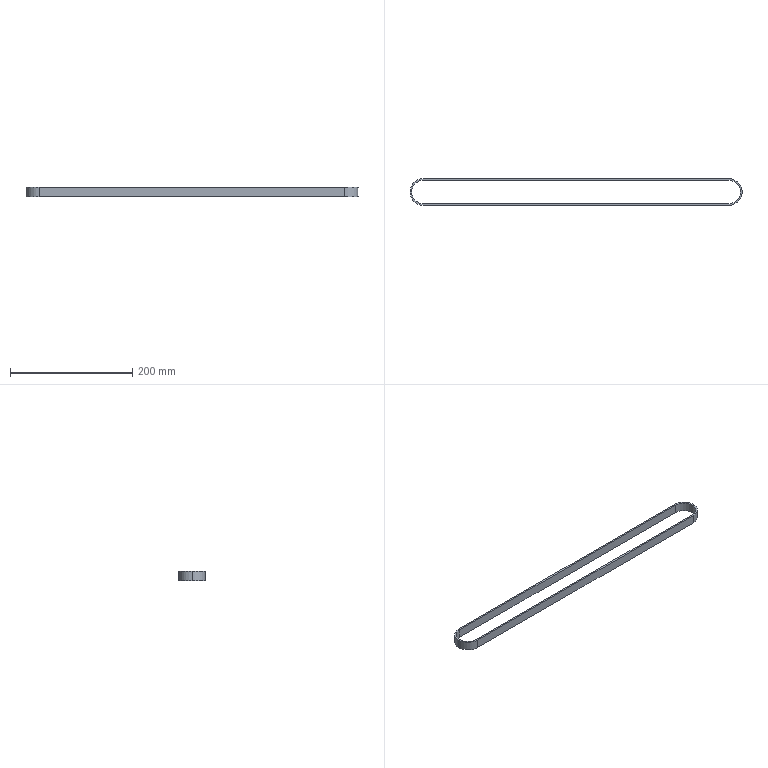Part | STEP file | Belt 1-2^ double-tube high-torque assembly | 1 solid | 12 faces | box 543.89 x 43.89 x 15 mm | volume 44395 mm3 | cylinder 6 | plane 6 | commonest cylinder face diameters 38.65 x3 43.89 x3
STEP:
#1=CARTESIAN_POINT('',(0.,0.,0.));
#2=DIRECTION('',(0.,0.,1.));
#3=DIRECTION('',(1.,0.,0.));
#4=AXIS2_PLACEMENT_3D('',#1,#2,#3);
#5=CARTESIAN_POINT('',(-14.086,14.168,15.));
#6=VERTEX_POINT('',#5);
#7=CARTESIAN_POINT('',(-14.086,14.168,0.));
#8=VERTEX_POINT('',#7);
#9=CARTESIAN_POINT('',(-14.086,14.168,15.));
#10=DIRECTION('',(0.,0.,-1.));
#11=VECTOR('',#10,1.);
#12=LINE('',#9,#11);
#13=CARTESIAN_POINT('',(-14.086,-5.157,15.));
#14=DIRECTION('',(0.,0.,-1.));
#15=DIRECTION('',(-1.,0.,0.));
#16=AXIS2_PLACEMENT_3D('',#13,#14,#15);
#17=CYLINDRICAL_SURFACE('',#16,19.325);
#18=CARTESIAN_POINT('',(1.571,0.));
#19=DIRECTION('',(0.,1.));
#20=VECTOR('',#19,1.);
#21=LINE('',#18,#20);
#22=(GEOMETRIC_REPRESENTATION_CONTEXT(2)PARAMETRIC_REPRESENTATION_CONTEXT()REPRESENTATION_CONTEXT('',''));
#23=DEFINITIONAL_REPRESENTATION('',(#21),#22);
#24=PCURVE('',#17,#23);
#25=CARTESIAN_POINT('',(-14.086,14.168,15.));
#26=DIRECTION('',(0.,1.,0.));
#27=DIRECTION('',(-1.,0.,0.));
#28=AXIS2_PLACEMENT_3D('',#25,#26,#27);
#29=PLANE('',#28);
#30=CARTESIAN_POINT('',(0.,0.));
#31=DIRECTION('',(0.,-1.));
#32=VECTOR('',#31,1.);
#33=LINE('',#30,#32);
#34=(GEOMETRIC_REPRESENTATION_CONTEXT(2)PARAMETRIC_REPRESENTATION_CONTEXT()REPRESENTATION_CONTEXT('',''));
#35=DEFINITIONAL_REPRESENTATION('',(#33),#34);
#36=PCURVE('',#29,#35);
#37=SURFACE_CURVE('',#12,(#24,#36),.PCURVE_S1.);
#38=EDGE_CURVE('',#6,#8,#37,.T.);
#39=ORIENTED_EDGE('',*,*,#38,.T.);
#40=CARTESIAN_POINT('',(-33.411,-5.157,0.));
#41=VERTEX_POINT('',#40);
#42=CARTESIAN_POINT('',(-14.086,-5.157,0.));
#43=DIRECTION('',(0.,0.,-1.));
#44=DIRECTION('',(-1.,0.,0.));
#45=AXIS2_PLACEMENT_3D('',#42,#43,#44);
#46=CIRCLE('',#45,19.325);
#47=CARTESIAN_POINT('',(0.,15.));
#48=DIRECTION('',(1.,0.));
#49=VECTOR('',#48,1.);
#50=LINE('',#47,#49);
#51=(GEOMETRIC_REPRESENTATION_CONTEXT(2)PARAMETRIC_REPRESENTATION_CONTEXT()REPRESENTATION_CONTEXT('',''));
#52=DEFINITIONAL_REPRESENTATION('',(#50),#51);
#53=PCURVE('',#17,#52);
#54=CARTESIAN_POINT('',(-14.086,-5.157,0.));
#55=DIRECTION('',(0.,0.,-1.));
#56=DIRECTION('',(-1.,0.,0.));
#57=AXIS2_PLACEMENT_3D('',#54,#55,#56);
#58=PLANE('',#57);
#59=CARTESIAN_POINT('',(0.,0.));
#60=DIRECTION('',(1.,0.));
#61=AXIS2_PLACEMENT_2D('',#59,#60);
#62=CIRCLE('',#61,19.325);
#63=(GEOMETRIC_REPRESENTATION_CONTEXT(2)PARAMETRIC_REPRESENTATION_CONTEXT()REPRESENTATION_CONTEXT('',''));
#64=DEFINITIONAL_REPRESENTATION('',(#62),#63);
#65=PCURVE('',#58,#64);
#66=SURFACE_CURVE('',#46,(#53,#65),.PCURVE_S1.);
#67=EDGE_CURVE('',#41,#8,#66,.T.);
#68=ORIENTED_EDGE('',*,*,#67,.F.);
#69=CARTESIAN_POINT('',(-33.411,-5.157,15.));
#70=VERTEX_POINT('',#69);
#71=CARTESIAN_POINT('',(-33.411,-5.157,15.));
#72=DIRECTION('',(0.,0.,-1.));
#73=VECTOR('',#72,1.);
#74=LINE('',#71,#73);
#75=CARTESIAN_POINT('',(0.,0.));
#76=DIRECTION('',(0.,1.));
#77=VECTOR('',#76,1.);
#78=LINE('',#75,#77);
#79=(GEOMETRIC_REPRESENTATION_CONTEXT(2)PARAMETRIC_REPRESENTATION_CONTEXT()REPRESENTATION_CONTEXT('',''));
#80=DEFINITIONAL_REPRESENTATION('',(#78),#79);
#81=PCURVE('',#17,#80);
#82=CARTESIAN_POINT('',(-14.086,-5.157,15.));
#83=DIRECTION('',(0.,0.,-1.));
#84=DIRECTION('',(-1.,0.,0.));
#85=AXIS2_PLACEMENT_3D('',#82,#83,#84);
#86=CYLINDRICAL_SURFACE('',#85,19.325);
#87=CARTESIAN_POINT('',(6.283,0.));
#88=DIRECTION('',(0.,1.));
#89=VECTOR('',#88,1.);
#90=LINE('',#87,#89);
#91=(GEOMETRIC_REPRESENTATION_CONTEXT(2)PARAMETRIC_REPRESENTATION_CONTEXT()REPRESENTATION_CONTEXT('',''));
#92=DEFINITIONAL_REPRESENTATION('',(#90),#91);
#93=PCURVE('',#86,#92);
#94=SURFACE_CURVE('',#74,(#81,#93),.PCURVE_S1.);
#95=EDGE_CURVE('',#70,#41,#94,.T.);
#96=ORIENTED_EDGE('',*,*,#95,.F.);
#97=CARTESIAN_POINT('',(-14.086,-5.157,15.));
#98=DIRECTION('',(0.,0.,-1.));
#99=DIRECTION('',(-1.,0.,0.));
#100=AXIS2_PLACEMENT_3D('',#97,#98,#99);
#101=CIRCLE('',#100,19.325);
#102=CARTESIAN_POINT('',(0.,0.));
#103=DIRECTION('',(1.,0.));
#104=VECTOR('',#103,1.);
#105=LINE('',#102,#104);
#106=(GEOMETRIC_REPRESENTATION_CONTEXT(2)PARAMETRIC_REPRESENTATION_CONTEXT()REPRESENTATION_CONTEXT('',''));
#107=DEFINITIONAL_REPRESENTATION('',(#105),#106);
#108=PCURVE('',#17,#107);
#109=CARTESIAN_POINT('',(-14.086,-5.157,15.));
#110=DIRECTION('',(0.,0.,-1.));
#111=DIRECTION('',(-1.,0.,0.));
#112=AXIS2_PLACEMENT_3D('',#109,#110,#111);
#113=PLANE('',#112);
#114=CARTESIAN_POINT('',(0.,0.));
#115=DIRECTION('',(1.,0.));
#116=AXIS2_PLACEMENT_2D('',#114,#115);
#117=CIRCLE('',#116,19.325);
#118=(GEOMETRIC_REPRESENTATION_CONTEXT(2)PARAMETRIC_REPRESENTATION_CONTEXT()REPRESENTATION_CONTEXT('',''));
#119=DEFINITIONAL_REPRESENTATION('',(#117),#118);
#120=PCURVE('',#113,#119);
#121=SURFACE_CURVE('',#101,(#108,#120),.PCURVE_S1.);
#122=EDGE_CURVE('',#70,#6,#121,.T.);
#123=ORIENTED_EDGE('',*,*,#122,.T.);
#124=EDGE_LOOP('',(#39,#68,#96,#123));
#125=FACE_BOUND('',#124,.F.);
#126=ADVANCED_FACE('',(#125),#17,.F.);
#127=CARTESIAN_POINT('',(-14.086,-27.102,15.));
#128=VERTEX_POINT('',#127);
#129=CARTESIAN_POINT('',(-36.031,-5.157,15.));
#130=VERTEX_POINT('',#129);
#131=CARTESIAN_POINT('',(-14.086,-5.157,15.));
#132=DIRECTION('',(0.,0.,-1.));
#133=DIRECTION('',(-1.,0.,0.));
#134=AXIS2_PLACEMENT_3D('',#131,#132,#133);
#135=CIRCLE('',#134,21.945);
#136=CARTESIAN_POINT('',(-14.086,-5.157,15.));
#137=DIRECTION('',(0.,0.,-1.));
#138=DIRECTION('',(-1.,0.,0.));
#139=AXIS2_PLACEMENT_3D('',#136,#137,#138);
#140=CYLINDRICAL_SURFACE('',#139,21.945);
#141=CARTESIAN_POINT('',(0.,0.));
#142=DIRECTION('',(1.,0.));
#143=VECTOR('',#142,1.);
#144=LINE('',#141,#143);
#145=(GEOMETRIC_REPRESENTATION_CONTEXT(2)PARAMETRIC_REPRESENTATION_CONTEXT()REPRESENTATION_CONTEXT('',''));
#146=DEFINITIONAL_REPRESENTATION('',(#144),#145);
#147=PCURVE('',#140,#146);
#148=CARTESIAN_POINT('',(0.,0.));
#149=DIRECTION('',(1.,0.));
#150=AXIS2_PLACEMENT_2D('',#148,#149);
#151=CIRCLE('',#150,21.945);
#152=(GEOMETRIC_REPRESENTATION_CONTEXT(2)PARAMETRIC_REPRESENTATION_CONTEXT()REPRESENTATION_CONTEXT('',''));
#153=DEFINITIONAL_REPRESENTATION('',(#151),#152);
#154=PCURVE('',#113,#153);
#155=SURFACE_CURVE('',#135,(#147,#154),.PCURVE_S1.);
#156=EDGE_CURVE('',#128,#130,#155,.T.);
#157=ORIENTED_EDGE('',*,*,#156,.T.);
#158=CARTESIAN_POINT('',(-36.031,-5.157,0.));
#159=VERTEX_POINT('',#158);
#160=CARTESIAN_POINT('',(-36.031,-5.157,15.));
#161=DIRECTION('',(0.,0.,-1.));
#162=VECTOR('',#161,1.);
#163=LINE('',#160,#162);
#164=CARTESIAN_POINT('',(6.283,0.));
#165=DIRECTION('',(0.,1.));
#166=VECTOR('',#165,1.);
#167=LINE('',#164,#166);
#168=(GEOMETRIC_REPRESENTATION_CONTEXT(2)PARAMETRIC_REPRESENTATION_CONTEXT()REPRESENTATION_CONTEXT('',''));
#169=DEFINITIONAL_REPRESENTATION('',(#167),#168);
#170=PCURVE('',#140,#169);
#171=CARTESIAN_POINT('',(-14.086,-5.157,15.));
#172=DIRECTION('',(0.,0.,-1.));
#173=DIRECTION('',(-1.,0.,0.));
#174=AXIS2_PLACEMENT_3D('',#171,#172,#173);
#175=CYLINDRICAL_SURFACE('',#174,21.945);
#176=CARTESIAN_POINT('',(0.,0.));
#177=DIRECTION('',(0.,1.));
#178=VECTOR('',#177,1.);
#179=LINE('',#176,#178);
#180=(GEOMETRIC_REPRESENTATION_CONTEXT(2)PARAMETRIC_REPRESENTATION_CONTEXT()REPRESENTATION_CONTEXT('',''));
#181=DEFINITIONAL_REPRESENTATION('',(#179),#180);
#182=PCURVE('',#175,#181);
#183=SURFACE_CURVE('',#163,(#170,#182),.PCURVE_S1.);
#184=EDGE_CURVE('',#130,#159,#183,.T.);
#185=ORIENTED_EDGE('',*,*,#184,.T.);
#186=CARTESIAN_POINT('',(-14.086,-27.102,0.));
#187=VERTEX_POINT('',#186);
#188=CARTESIAN_POINT('',(-14.086,-5.157,0.));
#189=DIRECTION('',(0.,0.,-1.));
#190=DIRECTION('',(-1.,0.,0.));
#191=AXIS2_PLACEMENT_3D('',#188,#189,#190);
#192=CIRCLE('',#191,21.945);
#193=CARTESIAN_POINT('',(0.,15.));
#194=DIRECTION('',(1.,0.));
#195=VECTOR('',#194,1.);
#196=LINE('',#193,#195);
#197=(GEOMETRIC_REPRESENTATION_CONTEXT(2)PARAMETRIC_REPRESENTATION_CONTEXT()REPRESENTATION_CONTEXT('',''));
#198=DEFINITIONAL_REPRESENTATION('',(#196),#197);
#199=PCURVE('',#140,#198);
#200=CARTESIAN_POINT('',(0.,0.));
#201=DIRECTION('',(1.,0.));
#202=AXIS2_PLACEMENT_2D('',#200,#201);
#203=CIRCLE('',#202,21.945);
#204=(GEOMETRIC_REPRESENTATION_CONTEXT(2)PARAMETRIC_REPRESENTATION_CONTEXT()REPRESENTATION_CONTEXT('',''));
#205=DEFINITIONAL_REPRESENTATION('',(#203),#204);
#206=PCURVE('',#58,#205);
#207=SURFACE_CURVE('',#192,(#199,#206),.PCURVE_S1.);
#208=EDGE_CURVE('',#187,#159,#207,.T.);
#209=ORIENTED_EDGE('',*,*,#208,.F.);
#210=CARTESIAN_POINT('',(-14.086,-27.102,15.));
#211=DIRECTION('',(0.,0.,-1.));
#212=VECTOR('',#211,1.);
#213=LINE('',#210,#212);
#214=CARTESIAN_POINT('',(4.712,0.));
#215=DIRECTION('',(0.,1.));
#216=VECTOR('',#215,1.);
#217=LINE('',#214,#216);
#218=(GEOMETRIC_REPRESENTATION_CONTEXT(2)PARAMETRIC_REPRESENTATION_CONTEXT()REPRESENTATION_CONTEXT('',''));
#219=DEFINITIONAL_REPRESENTATION('',(#217),#218);
#220=PCURVE('',#140,#219);
#221=CARTESIAN_POINT('',(-14.086,-27.102,15.));
#222=DIRECTION('',(0.,-1.,0.));
#223=DIRECTION('',(1.,0.,0.));
#224=AXIS2_PLACEMENT_3D('',#221,#222,#223);
#225=PLANE('',#224);
#226=CARTESIAN_POINT('',(0.,0.));
#227=DIRECTION('',(0.,-1.));
#228=VECTOR('',#227,1.);
#229=LINE('',#226,#228);
#230=(GEOMETRIC_REPRESENTATION_CONTEXT(2)PARAMETRIC_REPRESENTATION_CONTEXT()REPRESENTATION_CONTEXT('',''));
#231=DEFINITIONAL_REPRESENTATION('',(#229),#230);
#232=PCURVE('',#225,#231);
#233=SURFACE_CURVE('',#213,(#220,#232),.PCURVE_S1.);
#234=EDGE_CURVE('',#128,#187,#233,.T.);
#235=ORIENTED_EDGE('',*,*,#234,.F.);
#236=EDGE_LOOP('',(#157,#185,#209,#235));
#237=FACE_BOUND('',#236,.T.);
#238=ADVANCED_FACE('',(#237),#140,.T.);
#239=ORIENTED_EDGE('',*,*,#184,.F.);
#240=CARTESIAN_POINT('',(-14.086,16.788,15.));
#241=VERTEX_POINT('',#240);
#242=CARTESIAN_POINT('',(-14.086,-5.157,15.));
#243=DIRECTION('',(0.,0.,-1.));
#244=DIRECTION('',(-1.,0.,0.));
#245=AXIS2_PLACEMENT_3D('',#242,#243,#244);
#246=CIRCLE('',#245,21.945);
#247=CARTESIAN_POINT('',(0.,0.));
#248=DIRECTION('',(1.,0.));
#249=VECTOR('',#248,1.);
#250=LINE('',#247,#249);
#251=(GEOMETRIC_REPRESENTATION_CONTEXT(2)PARAMETRIC_REPRESENTATION_CONTEXT()REPRESENTATION_CONTEXT('',''));
#252=DEFINITIONAL_REPRESENTATION('',(#250),#251);
#253=PCURVE('',#175,#252);
#254=CARTESIAN_POINT('',(0.,0.));
#255=DIRECTION('',(1.,0.));
#256=AXIS2_PLACEMENT_2D('',#254,#255);
#257=CIRCLE('',#256,21.945);
#258=(GEOMETRIC_REPRESENTATION_CONTEXT(2)PARAMETRIC_REPRESENTATION_CONTEXT()REPRESENTATION_CONTEXT('',''));
#259=DEFINITIONAL_REPRESENTATION('',(#257),#258);
#260=PCURVE('',#113,#259);
#261=SURFACE_CURVE('',#246,(#253,#260),.PCURVE_S1.);
#262=EDGE_CURVE('',#130,#241,#261,.T.);
#263=ORIENTED_EDGE('',*,*,#262,.T.);
#264=CARTESIAN_POINT('',(-14.086,16.788,0.));
#265=VERTEX_POINT('',#264);
#266=CARTESIAN_POINT('',(-14.086,16.788,15.));
#267=DIRECTION('',(0.,0.,-1.));
#268=VECTOR('',#267,1.);
#269=LINE('',#266,#268);
#270=CARTESIAN_POINT('',(1.571,0.));
#271=DIRECTION('',(0.,1.));
#272=VECTOR('',#271,1.);
#273=LINE('',#270,#272);
#274=(GEOMETRIC_REPRESENTATION_CONTEXT(2)PARAMETRIC_REPRESENTATION_CONTEXT()REPRESENTATION_CONTEXT('',''));
#275=DEFINITIONAL_REPRESENTATION('',(#273),#274);
#276=PCURVE('',#175,#275);
#277=CARTESIAN_POINT('',(-14.086,16.788,15.));
#278=DIRECTION('',(0.,1.,0.));
#279=DIRECTION('',(-1.,0.,0.));
#280=AXIS2_PLACEMENT_3D('',#277,#278,#279);
#281=PLANE('',#280);
#282=CARTESIAN_POINT('',(0.,0.));
#283=DIRECTION('',(0.,-1.));
#284=VECTOR('',#283,1.);
#285=LINE('',#282,#284);
#286=(GEOMETRIC_REPRESENTATION_CONTEXT(2)PARAMETRIC_REPRESENTATION_CONTEXT()REPRESENTATION_CONTEXT('',''));
#287=DEFINITIONAL_REPRESENTATION('',(#285),#286);
#288=PCURVE('',#281,#287);
#289=SURFACE_CURVE('',#269,(#276,#288),.PCURVE_S1.);
#290=EDGE_CURVE('',#241,#265,#289,.T.);
#291=ORIENTED_EDGE('',*,*,#290,.T.);
#292=CARTESIAN_POINT('',(-14.086,-5.157,0.));
#293=DIRECTION('',(0.,0.,-1.));
#294=DIRECTION('',(-1.,0.,0.));
#295=AXIS2_PLACEMENT_3D('',#292,#293,#294);
#296=CIRCLE('',#295,21.945);
#297=CARTESIAN_POINT('',(0.,15.));
#298=DIRECTION('',(1.,0.));
#299=VECTOR('',#298,1.);
#300=LINE('',#297,#299);
#301=(GEOMETRIC_REPRESENTATION_CONTEXT(2)PARAMETRIC_REPRESENTATION_CONTEXT()REPRESENTATION_CONTEXT('',''));
#302=DEFINITIONAL_REPRESENTATION('',(#300),#301);
#303=PCURVE('',#175,#302);
#304=CARTESIAN_POINT('',(0.,0.));
#305=DIRECTION('',(1.,0.));
#306=AXIS2_PLACEMENT_2D('',#304,#305);
#307=CIRCLE('',#306,21.945);
#308=(GEOMETRIC_REPRESENTATION_CONTEXT(2)PARAMETRIC_REPRESENTATION_CONTEXT()REPRESENTATION_CONTEXT('',''));
#309=DEFINITIONAL_REPRESENTATION('',(#307),#308);
#310=PCURVE('',#58,#309);
#311=SURFACE_CURVE('',#296,(#303,#310),.PCURVE_S1.);
#312=EDGE_CURVE('',#159,#265,#311,.T.);
#313=ORIENTED_EDGE('',*,*,#312,.F.);
#314=EDGE_LOOP('',(#239,#263,#291,#313));
#315=FACE_BOUND('',#314,.T.);
#316=ADVANCED_FACE('',(#315),#175,.T.);
#317=CARTESIAN_POINT('',(485.914,-27.102,0.));
#318=VERTEX_POINT('',#317);
#319=CARTESIAN_POINT('',(-14.086,-27.102,0.));
#320=DIRECTION('',(-1.,0.,0.));
#321=VECTOR('',#320,1.);
#322=LINE('',#319,#321);
#323=CARTESIAN_POINT('',(0.,-15.));
#324=DIRECTION('',(-1.,0.));
#325=VECTOR('',#324,1.);
#326=LINE('',#323,#325);
#327=(GEOMETRIC_REPRESENTATION_CONTEXT(2)PARAMETRIC_REPRESENTATION_CONTEXT()REPRESENTATION_CONTEXT('',''));
#328=DEFINITIONAL_REPRESENTATION('',(#326),#327);
#329=PCURVE('',#225,#328);
#330=CARTESIAN_POINT('',(0.,-21.945));
#331=DIRECTION('',(1.,0.));
#332=VECTOR('',#331,1.);
#333=LINE('',#330,#332);
#334=(GEOMETRIC_REPRESENTATION_CONTEXT(2)PARAMETRIC_REPRESENTATION_CONTEXT()REPRESENTATION_CONTEXT('',''));
#335=DEFINITIONAL_REPRESENTATION('',(#333),#334);
#336=PCURVE('',#58,#335);
#337=SURFACE_CURVE('',#322,(#329,#336),.PCURVE_S1.);
#338=EDGE_CURVE('',#318,#187,#337,.T.);
#339=ORIENTED_EDGE('',*,*,#338,.F.);
#340=CARTESIAN_POINT('',(485.914,-27.102,15.));
#341=VERTEX_POINT('',#340);
#342=CARTESIAN_POINT('',(485.914,-27.102,15.));
#343=DIRECTION('',(0.,0.,-1.));
#344=VECTOR('',#343,1.);
#345=LINE('',#342,#344);
#346=CARTESIAN_POINT('',(500.,0.));
#347=DIRECTION('',(0.,-1.));
#348=VECTOR('',#347,1.);
#349=LINE('',#346,#348);
#350=(GEOMETRIC_REPRESENTATION_CONTEXT(2)PARAMETRIC_REPRESENTATION_CONTEXT()REPRESENTATION_CONTEXT('',''));
#351=DEFINITIONAL_REPRESENTATION('',(#349),#350);
#352=PCURVE('',#225,#351);
#353=CARTESIAN_POINT('',(485.914,-5.157,15.));
#354=DIRECTION('',(0.,0.,-1.));
#355=DIRECTION('',(-1.,0.,0.));
#356=AXIS2_PLACEMENT_3D('',#353,#354,#355);
#357=CYLINDRICAL_SURFACE('',#356,21.945);
#358=CARTESIAN_POINT('',(4.712,0.));
#359=DIRECTION('',(0.,1.));
#360=VECTOR('',#359,1.);
#361=LINE('',#358,#360);
#362=(GEOMETRIC_REPRESENTATION_CONTEXT(2)PARAMETRIC_REPRESENTATION_CONTEXT()REPRESENTATION_CONTEXT('',''));
#363=DEFINITIONAL_REPRESENTATION('',(#361),#362);
#364=PCURVE('',#357,#363);
#365=SURFACE_CURVE('',#345,(#352,#364),.PCURVE_S1.);
#366=EDGE_CURVE('',#341,#318,#365,.T.);
#367=ORIENTED_EDGE('',*,*,#366,.F.);
#368=CARTESIAN_POINT('',(-14.086,-27.102,15.));
#369=DIRECTION('',(-1.,0.,0.));
#370=VECTOR('',#369,1.);
#371=LINE('',#368,#370);
#372=CARTESIAN_POINT('',(0.,0.));
#373=DIRECTION('',(-1.,0.));
#374=VECTOR('',#373,1.);
#375=LINE('',#372,#374);
#376=(GEOMETRIC_REPRESENTATION_CONTEXT(2)PARAMETRIC_REPRESENTATION_CONTEXT()REPRESENTATION_CONTEXT('',''));
#377=DEFINITIONAL_REPRESENTATION('',(#375),#376);
#378=PCURVE('',#225,#377);
#379=CARTESIAN_POINT('',(0.,-21.945));
#380=DIRECTION('',(1.,0.));
#381=VECTOR('',#380,1.);
#382=LINE('',#379,#381);
#383=(GEOMETRIC_REPRESENTATION_CONTEXT(2)PARAMETRIC_REPRESENTATION_CONTEXT()REPRESENTATION_CONTEXT('',''));
#384=DEFINITIONAL_REPRESENTATION('',(#382),#383);
#385=PCURVE('',#113,#384);
#386=SURFACE_CURVE('',#371,(#378,#385),.PCURVE_S1.);
#387=EDGE_CURVE('',#341,#128,#386,.T.);
#388=ORIENTED_EDGE('',*,*,#387,.T.);
#389=ORIENTED_EDGE('',*,*,#234,.T.);
#390=EDGE_LOOP('',(#339,#367,#388,#389));
#391=FACE_BOUND('',#390,.T.);
#392=ADVANCED_FACE('',(#391),#225,.T.);
#393=CARTESIAN_POINT('',(485.914,16.788,0.));
#394=VERTEX_POINT('',#393);
#395=CARTESIAN_POINT('',(485.914,-5.157,0.));
#396=DIRECTION('',(0.,0.,-1.));
#397=DIRECTION('',(-1.,0.,0.));
#398=AXIS2_PLACEMENT_3D('',#395,#396,#397);
#399=CIRCLE('',#398,21.945);
#400=CARTESIAN_POINT('',(0.,15.));
#401=DIRECTION('',(1.,0.));
#402=VECTOR('',#401,1.);
#403=LINE('',#400,#402);
#404=(GEOMETRIC_REPRESENTATION_CONTEXT(2)PARAMETRIC_REPRESENTATION_CONTEXT()REPRESENTATION_CONTEXT('',''));
#405=DEFINITIONAL_REPRESENTATION('',(#403),#404);
#406=PCURVE('',#357,#405);
#407=CARTESIAN_POINT('',(-500.,0.));
#408=DIRECTION('',(1.,0.));
#409=AXIS2_PLACEMENT_2D('',#407,#408);
#410=CIRCLE('',#409,21.945);
#411=(GEOMETRIC_REPRESENTATION_CONTEXT(2)PARAMETRIC_REPRESENTATION_CONTEXT()REPRESENTATION_CONTEXT('',''));
#412=DEFINITIONAL_REPRESENTATION('',(#410),#411);
#413=PCURVE('',#58,#412);
#414=SURFACE_CURVE('',#399,(#406,#413),.PCURVE_S1.);
#415=EDGE_CURVE('',#394,#318,#414,.T.);
#416=ORIENTED_EDGE('',*,*,#415,.F.);
#417=CARTESIAN_POINT('',(485.914,16.788,15.));
#418=VERTEX_POINT('',#417);
#419=CARTESIAN_POINT('',(485.914,16.788,15.));
#420=DIRECTION('',(0.,0.,-1.));
#421=VECTOR('',#420,1.);
#422=LINE('',#419,#421);
#423=CARTESIAN_POINT('',(1.571,0.));
#424=DIRECTION('',(0.,1.));
#425=VECTOR('',#424,1.);
#426=LINE('',#423,#425);
#427=(GEOMETRIC_REPRESENTATION_CONTEXT(2)PARAMETRIC_REPRESENTATION_CONTEXT()REPRESENTATION_CONTEXT('',''));
#428=DEFINITIONAL_REPRESENTATION('',(#426),#427);
#429=PCURVE('',#357,#428);
#430=CARTESIAN_POINT('',(-500.,0.));
#431=DIRECTION('',(0.,-1.));
#432=VECTOR('',#431,1.);
#433=LINE('',#430,#432);
#434=(GEOMETRIC_REPRESENTATION_CONTEXT(2)PARAMETRIC_REPRESENTATION_CONTEXT()REPRESENTATION_CONTEXT('',''));
#435=DEFINITIONAL_REPRESENTATION('',(#433),#434);
#436=PCURVE('',#281,#435);
#437=SURFACE_CURVE('',#422,(#429,#436),.PCURVE_S1.);
#438=EDGE_CURVE('',#418,#394,#437,.T.);
#439=ORIENTED_EDGE('',*,*,#438,.F.);
#440=CARTESIAN_POINT('',(485.914,-5.157,15.));
#441=DIRECTION('',(0.,0.,-1.));
#442=DIRECTION('',(-1.,0.,0.));
#443=AXIS2_PLACEMENT_3D('',#440,#441,#442);
#444=CIRCLE('',#443,21.945);
#445=CARTESIAN_POINT('',(0.,0.));
#446=DIRECTION('',(1.,0.));
#447=VECTOR('',#446,1.);
#448=LINE('',#445,#447);
#449=(GEOMETRIC_REPRESENTATION_CONTEXT(2)PARAMETRIC_REPRESENTATION_CONTEXT()REPRESENTATION_CONTEXT('',''));
#450=DEFINITIONAL_REPRESENTATION('',(#448),#449);
#451=PCURVE('',#357,#450);
#452=CARTESIAN_POINT('',(-500.,0.));
#453=DIRECTION('',(1.,0.));
#454=AXIS2_PLACEMENT_2D('',#452,#453);
#455=CIRCLE('',#454,21.945);
#456=(GEOMETRIC_REPRESENTATION_CONTEXT(2)PARAMETRIC_REPRESENTATION_CONTEXT()REPRESENTATION_CONTEXT('',''));
#457=DEFINITIONAL_REPRESENTATION('',(#455),#456);
#458=PCURVE('',#113,#457);
#459=SURFACE_CURVE('',#444,(#451,#458),.PCURVE_S1.);
#460=EDGE_CURVE('',#418,#341,#459,.T.);
#461=ORIENTED_EDGE('',*,*,#460,.T.);
#462=ORIENTED_EDGE('',*,*,#366,.T.);
#463=EDGE_LOOP('',(#416,#439,#461,#462));
#464=FACE_BOUND('',#463,.T.);
#465=ADVANCED_FACE('',(#464),#357,.T.);
#466=CARTESIAN_POINT('',(-14.086,16.788,0.));
#467=DIRECTION('',(1.,0.,0.));
#468=VECTOR('',#467,1.);
#469=LINE('',#466,#468);
#470=CARTESIAN_POINT('',(0.,-15.));
#471=DIRECTION('',(-1.,0.));
#472=VECTOR('',#471,1.);
#473=LINE('',#470,#472);
#474=(GEOMETRIC_REPRESENTATION_CONTEXT(2)PARAMETRIC_REPRESENTATION_CONTEXT()REPRESENTATION_CONTEXT('',''));
#475=DEFINITIONAL_REPRESENTATION('',(#473),#474);
#476=PCURVE('',#281,#475);
#477=CARTESIAN_POINT('',(0.,21.945));
#478=DIRECTION('',(-1.,0.));
#479=VECTOR('',#478,1.);
#480=LINE('',#477,#479);
#481=(GEOMETRIC_REPRESENTATION_CONTEXT(2)PARAMETRIC_REPRESENTATION_CONTEXT()REPRESENTATION_CONTEXT('',''));
#482=DEFINITIONAL_REPRESENTATION('',(#480),#481);
#483=PCURVE('',#58,#482);
#484=SURFACE_CURVE('',#469,(#476,#483),.PCURVE_S1.);
#485=EDGE_CURVE('',#265,#394,#484,.T.);
#486=ORIENTED_EDGE('',*,*,#485,.F.);
#487=ORIENTED_EDGE('',*,*,#290,.F.);
#488=CARTESIAN_POINT('',(-14.086,16.788,15.));
#489=DIRECTION('',(1.,0.,0.));
#490=VECTOR('',#489,1.);
#491=LINE('',#488,#490);
#492=CARTESIAN_POINT('',(0.,0.));
#493=DIRECTION('',(-1.,0.));
#494=VECTOR('',#493,1.);
#495=LINE('',#492,#494);
#496=(GEOMETRIC_REPRESENTATION_CONTEXT(2)PARAMETRIC_REPRESENTATION_CONTEXT()REPRESENTATION_CONTEXT('',''));
#497=DEFINITIONAL_REPRESENTATION('',(#495),#496);
#498=PCURVE('',#281,#497);
#499=CARTESIAN_POINT('',(0.,21.945));
#500=DIRECTION('',(-1.,0.));
#501=VECTOR('',#500,1.);
#502=LINE('',#499,#501);
#503=(GEOMETRIC_REPRESENTATION_CONTEXT(2)PARAMETRIC_REPRESENTATION_CONTEXT()REPRESENTATION_CONTEXT('',''));
#504=DEFINITIONAL_REPRESENTATION('',(#502),#503);
#505=PCURVE('',#113,#504);
#506=SURFACE_CURVE('',#491,(#498,#505),.PCURVE_S1.);
#507=EDGE_CURVE('',#241,#418,#506,.T.);
#508=ORIENTED_EDGE('',*,*,#507,.T.);
#509=ORIENTED_EDGE('',*,*,#438,.T.);
#510=EDGE_LOOP('',(#486,#487,#508,#509));
#511=FACE_BOUND('',#510,.T.);
#512=ADVANCED_FACE('',(#511),#281,.T.);
#513=CARTESIAN_POINT('',(485.914,-24.482,15.));
#514=VERTEX_POINT('',#513);
#515=CARTESIAN_POINT('',(-14.086,-24.482,15.));
#516=VERTEX_POINT('',#515);
#517=CARTESIAN_POINT('',(485.914,-24.482,15.));
#518=DIRECTION('',(-1.,0.,0.));
#519=VECTOR('',#518,1.);
#520=LINE('',#517,#519);
#521=CARTESIAN_POINT('',(-500.,-19.325));
#522=DIRECTION('',(1.,0.));
#523=VECTOR('',#522,1.);
#524=LINE('',#521,#523);
#525=(GEOMETRIC_REPRESENTATION_CONTEXT(2)PARAMETRIC_REPRESENTATION_CONTEXT()REPRESENTATION_CONTEXT('',''));
#526=DEFINITIONAL_REPRESENTATION('',(#524),#525);
#527=PCURVE('',#113,#526);
#528=CARTESIAN_POINT('',(485.914,-24.482,15.));
#529=DIRECTION('',(0.,-1.,0.));
#530=DIRECTION('',(1.,0.,0.));
#531=AXIS2_PLACEMENT_3D('',#528,#529,#530);
#532=PLANE('',#531);
#533=CARTESIAN_POINT('',(0.,0.));
#534=DIRECTION('',(-1.,0.));
#535=VECTOR('',#534,1.);
#536=LINE('',#533,#535);
#537=(GEOMETRIC_REPRESENTATION_CONTEXT(2)PARAMETRIC_REPRESENTATION_CONTEXT()REPRESENTATION_CONTEXT('',''));
#538=DEFINITIONAL_REPRESENTATION('',(#536),#537);
#539=PCURVE('',#532,#538);
#540=SURFACE_CURVE('',#520,(#527,#539),.PCURVE_S1.);
#541=EDGE_CURVE('',#514,#516,#540,.T.);
#542=ORIENTED_EDGE('',*,*,#541,.T.);
#543=CARTESIAN_POINT('',(-14.086,-5.157,15.));
#544=DIRECTION('',(0.,0.,-1.));
#545=DIRECTION('',(-1.,0.,0.));
#546=AXIS2_PLACEMENT_3D('',#543,#544,#545);
#547=CIRCLE('',#546,19.325);
#548=CARTESIAN_POINT('',(0.,0.));
#549=DIRECTION('',(1.,0.));
#550=AXIS2_PLACEMENT_2D('',#548,#549);
#551=CIRCLE('',#550,19.325);
#552=(GEOMETRIC_REPRESENTATION_CONTEXT(2)PARAMETRIC_REPRESENTATION_CONTEXT()REPRESENTATION_CONTEXT('',''));
#553=DEFINITIONAL_REPRESENTATION('',(#551),#552);
#554=PCURVE('',#113,#553);
#555=CARTESIAN_POINT('',(0.,0.));
#556=DIRECTION('',(1.,0.));
#557=VECTOR('',#556,1.);
#558=LINE('',#555,#557);
#559=(GEOMETRIC_REPRESENTATION_CONTEXT(2)PARAMETRIC_REPRESENTATION_CONTEXT()REPRESENTATION_CONTEXT('',''));
#560=DEFINITIONAL_REPRESENTATION('',(#558),#559);
#561=PCURVE('',#86,#560);
#562=SURFACE_CURVE('',#547,(#554,#561),.PCURVE_S1.);
#563=EDGE_CURVE('',#516,#70,#562,.T.);
#564=ORIENTED_EDGE('',*,*,#563,.T.);
#565=ORIENTED_EDGE('',*,*,#122,.T.);
#566=CARTESIAN_POINT('',(485.914,14.168,15.));
#567=VERTEX_POINT('',#566);
#568=CARTESIAN_POINT('',(-14.086,14.168,15.));
#569=DIRECTION('',(1.,0.,0.));
#570=VECTOR('',#569,1.);
#571=LINE('',#568,#570);
#572=CARTESIAN_POINT('',(0.,19.325));
#573=DIRECTION('',(-1.,0.));
#574=VECTOR('',#573,1.);
#575=LINE('',#572,#574);
#576=(GEOMETRIC_REPRESENTATION_CONTEXT(2)PARAMETRIC_REPRESENTATION_CONTEXT()REPRESENTATION_CONTEXT('',''));
#577=DEFINITIONAL_REPRESENTATION('',(#575),#576);
#578=PCURVE('',#113,#577);
#579=CARTESIAN_POINT('',(0.,0.));
#580=DIRECTION('',(-1.,0.));
#581=VECTOR('',#580,1.);
#582=LINE('',#579,#581);
#583=(GEOMETRIC_REPRESENTATION_CONTEXT(2)PARAMETRIC_REPRESENTATION_CONTEXT()REPRESENTATION_CONTEXT('',''));
#584=DEFINITIONAL_REPRESENTATION('',(#582),#583);
#585=PCURVE('',#29,#584);
#586=SURFACE_CURVE('',#571,(#578,#585),.PCURVE_S1.);
#587=EDGE_CURVE('',#6,#567,#586,.T.);
#588=ORIENTED_EDGE('',*,*,#587,.T.);
#589=CARTESIAN_POINT('',(485.914,-5.157,15.));
#590=DIRECTION('',(0.,0.,-1.));
#591=DIRECTION('',(-1.,0.,0.));
#592=AXIS2_PLACEMENT_3D('',#589,#590,#591);
#593=CIRCLE('',#592,19.325);
#594=CARTESIAN_POINT('',(-500.,0.));
#595=DIRECTION('',(1.,0.));
#596=AXIS2_PLACEMENT_2D('',#594,#595);
#597=CIRCLE('',#596,19.325);
#598=(GEOMETRIC_REPRESENTATION_CONTEXT(2)PARAMETRIC_REPRESENTATION_CONTEXT()REPRESENTATION_CONTEXT('',''));
#599=DEFINITIONAL_REPRESENTATION('',(#597),#598);
#600=PCURVE('',#113,#599);
#601=CARTESIAN_POINT('',(485.914,-5.157,15.));
#602=DIRECTION('',(0.,0.,-1.));
#603=DIRECTION('',(-1.,0.,0.));
#604=AXIS2_PLACEMENT_3D('',#601,#602,#603);
#605=CYLINDRICAL_SURFACE('',#604,19.325);
#606=CARTESIAN_POINT('',(0.,0.));
#607=DIRECTION('',(1.,0.));
#608=VECTOR('',#607,1.);
#609=LINE('',#606,#608);
#610=(GEOMETRIC_REPRESENTATION_CONTEXT(2)PARAMETRIC_REPRESENTATION_CONTEXT()REPRESENTATION_CONTEXT('',''));
#611=DEFINITIONAL_REPRESENTATION('',(#609),#610);
#612=PCURVE('',#605,#611);
#613=SURFACE_CURVE('',#593,(#600,#612),.PCURVE_S1.);
#614=EDGE_CURVE('',#567,#514,#613,.T.);
#615=ORIENTED_EDGE('',*,*,#614,.T.);
#616=EDGE_LOOP('',(#542,#564,#565,#588,#615));
#617=FACE_BOUND('',#616,.T.);
#618=ORIENTED_EDGE('',*,*,#156,.F.);
#619=ORIENTED_EDGE('',*,*,#387,.F.);
#620=ORIENTED_EDGE('',*,*,#460,.F.);
#621=ORIENTED_EDGE('',*,*,#507,.F.);
#622=ORIENTED_EDGE('',*,*,#262,.F.);
#623=EDGE_LOOP('',(#618,#619,#620,#621,#622));
#624=FACE_BOUND('',#623,.T.);
#625=ADVANCED_FACE('',(#617,#624),#113,.F.);
#626=CARTESIAN_POINT('',(-14.086,-24.482,0.));
#627=VERTEX_POINT('',#626);
#628=CARTESIAN_POINT('',(-14.086,-5.157,0.));
#629=DIRECTION('',(0.,0.,-1.));
#630=DIRECTION('',(-1.,0.,0.));
#631=AXIS2_PLACEMENT_3D('',#628,#629,#630);
#632=CIRCLE('',#631,19.325);
#633=CARTESIAN_POINT('',(0.,0.));
#634=DIRECTION('',(1.,0.));
#635=AXIS2_PLACEMENT_2D('',#633,#634);
#636=CIRCLE('',#635,19.325);
#637=(GEOMETRIC_REPRESENTATION_CONTEXT(2)PARAMETRIC_REPRESENTATION_CONTEXT()REPRESENTATION_CONTEXT('',''));
#638=DEFINITIONAL_REPRESENTATION('',(#636),#637);
#639=PCURVE('',#58,#638);
#640=CARTESIAN_POINT('',(0.,15.));
#641=DIRECTION('',(1.,0.));
#642=VECTOR('',#641,1.);
#643=LINE('',#640,#642);
#644=(GEOMETRIC_REPRESENTATION_CONTEXT(2)PARAMETRIC_REPRESENTATION_CONTEXT()REPRESENTATION_CONTEXT('',''));
#645=DEFINITIONAL_REPRESENTATION('',(#643),#644);
#646=PCURVE('',#86,#645);
#647=SURFACE_CURVE('',#632,(#639,#646),.PCURVE_S1.);
#648=EDGE_CURVE('',#627,#41,#647,.T.);
#649=ORIENTED_EDGE('',*,*,#648,.F.);
#650=CARTESIAN_POINT('',(485.914,-24.482,0.));
#651=VERTEX_POINT('',#650);
#652=CARTESIAN_POINT('',(485.914,-24.482,0.));
#653=DIRECTION('',(-1.,0.,0.));
#654=VECTOR('',#653,1.);
#655=LINE('',#652,#654);
#656=CARTESIAN_POINT('',(-500.,-19.325));
#657=DIRECTION('',(1.,0.));
#658=VECTOR('',#657,1.);
#659=LINE('',#656,#658);
#660=(GEOMETRIC_REPRESENTATION_CONTEXT(2)PARAMETRIC_REPRESENTATION_CONTEXT()REPRESENTATION_CONTEXT('',''));
#661=DEFINITIONAL_REPRESENTATION('',(#659),#660);
#662=PCURVE('',#58,#661);
#663=CARTESIAN_POINT('',(0.,-15.));
#664=DIRECTION('',(-1.,0.));
#665=VECTOR('',#664,1.);
#666=LINE('',#663,#665);
#667=(GEOMETRIC_REPRESENTATION_CONTEXT(2)PARAMETRIC_REPRESENTATION_CONTEXT()REPRESENTATION_CONTEXT('',''));
#668=DEFINITIONAL_REPRESENTATION('',(#666),#667);
#669=PCURVE('',#532,#668);
#670=SURFACE_CURVE('',#655,(#662,#669),.PCURVE_S1.);
#671=EDGE_CURVE('',#651,#627,#670,.T.);
#672=ORIENTED_EDGE('',*,*,#671,.F.);
#673=CARTESIAN_POINT('',(485.914,14.168,0.));
#674=VERTEX_POINT('',#673);
#675=CARTESIAN_POINT('',(485.914,-5.157,0.));
#676=DIRECTION('',(0.,0.,-1.));
#677=DIRECTION('',(-1.,0.,0.));
#678=AXIS2_PLACEMENT_3D('',#675,#676,#677);
#679=CIRCLE('',#678,19.325);
#680=CARTESIAN_POINT('',(-500.,0.));
#681=DIRECTION('',(1.,0.));
#682=AXIS2_PLACEMENT_2D('',#680,#681);
#683=CIRCLE('',#682,19.325);
#684=(GEOMETRIC_REPRESENTATION_CONTEXT(2)PARAMETRIC_REPRESENTATION_CONTEXT()REPRESENTATION_CONTEXT('',''));
#685=DEFINITIONAL_REPRESENTATION('',(#683),#684);
#686=PCURVE('',#58,#685);
#687=CARTESIAN_POINT('',(0.,15.));
#688=DIRECTION('',(1.,0.));
#689=VECTOR('',#688,1.);
#690=LINE('',#687,#689);
#691=(GEOMETRIC_REPRESENTATION_CONTEXT(2)PARAMETRIC_REPRESENTATION_CONTEXT()REPRESENTATION_CONTEXT('',''));
#692=DEFINITIONAL_REPRESENTATION('',(#690),#691);
#693=PCURVE('',#605,#692);
#694=SURFACE_CURVE('',#679,(#686,#693),.PCURVE_S1.);
#695=EDGE_CURVE('',#674,#651,#694,.T.);
#696=ORIENTED_EDGE('',*,*,#695,.F.);
#697=CARTESIAN_POINT('',(-14.086,14.168,0.));
#698=DIRECTION('',(1.,0.,0.));
#699=VECTOR('',#698,1.);
#700=LINE('',#697,#699);
#701=CARTESIAN_POINT('',(0.,19.325));
#702=DIRECTION('',(-1.,0.));
#703=VECTOR('',#702,1.);
#704=LINE('',#701,#703);
#705=(GEOMETRIC_REPRESENTATION_CONTEXT(2)PARAMETRIC_REPRESENTATION_CONTEXT()REPRESENTATION_CONTEXT('',''));
#706=DEFINITIONAL_REPRESENTATION('',(#704),#705);
#707=PCURVE('',#58,#706);
#708=CARTESIAN_POINT('',(0.,-15.));
#709=DIRECTION('',(-1.,0.));
#710=VECTOR('',#709,1.);
#711=LINE('',#708,#710);
#712=(GEOMETRIC_REPRESENTATION_CONTEXT(2)PARAMETRIC_REPRESENTATION_CONTEXT()REPRESENTATION_CONTEXT('',''));
#713=DEFINITIONAL_REPRESENTATION('',(#711),#712);
#714=PCURVE('',#29,#713);
#715=SURFACE_CURVE('',#700,(#707,#714),.PCURVE_S1.);
#716=EDGE_CURVE('',#8,#674,#715,.T.);
#717=ORIENTED_EDGE('',*,*,#716,.F.);
#718=ORIENTED_EDGE('',*,*,#67,.F.);
#719=EDGE_LOOP('',(#649,#672,#696,#717,#718));
#720=FACE_BOUND('',#719,.T.);
#721=ORIENTED_EDGE('',*,*,#208,.T.);
#722=ORIENTED_EDGE('',*,*,#312,.T.);
#723=ORIENTED_EDGE('',*,*,#485,.T.);
#724=ORIENTED_EDGE('',*,*,#415,.T.);
#725=ORIENTED_EDGE('',*,*,#338,.T.);
#726=EDGE_LOOP('',(#721,#722,#723,#724,#725));
#727=FACE_BOUND('',#726,.T.);
#728=ADVANCED_FACE('',(#720,#727),#58,.T.);
#729=ORIENTED_EDGE('',*,*,#648,.F.);
#730=CARTESIAN_POINT('',(-14.086,-24.482,15.));
#731=DIRECTION('',(0.,0.,-1.));
#732=VECTOR('',#731,1.);
#733=LINE('',#730,#732);
#734=CARTESIAN_POINT('',(4.712,0.));
#735=DIRECTION('',(0.,1.));
#736=VECTOR('',#735,1.);
#737=LINE('',#734,#736);
#738=(GEOMETRIC_REPRESENTATION_CONTEXT(2)PARAMETRIC_REPRESENTATION_CONTEXT()REPRESENTATION_CONTEXT('',''));
#739=DEFINITIONAL_REPRESENTATION('',(#737),#738);
#740=PCURVE('',#86,#739);
#741=CARTESIAN_POINT('',(-500.,0.));
#742=DIRECTION('',(0.,-1.));
#743=VECTOR('',#742,1.);
#744=LINE('',#741,#743);
#745=(GEOMETRIC_REPRESENTATION_CONTEXT(2)PARAMETRIC_REPRESENTATION_CONTEXT()REPRESENTATION_CONTEXT('',''));
#746=DEFINITIONAL_REPRESENTATION('',(#744),#745);
#747=PCURVE('',#532,#746);
#748=SURFACE_CURVE('',#733,(#740,#747),.PCURVE_S1.);
#749=EDGE_CURVE('',#516,#627,#748,.T.);
#750=ORIENTED_EDGE('',*,*,#749,.F.);
#751=ORIENTED_EDGE('',*,*,#563,.T.);
#752=ORIENTED_EDGE('',*,*,#95,.T.);
#753=EDGE_LOOP('',(#729,#750,#751,#752));
#754=FACE_BOUND('',#753,.F.);
#755=ADVANCED_FACE('',(#754),#86,.F.);
#756=ORIENTED_EDGE('',*,*,#671,.T.);
#757=ORIENTED_EDGE('',*,*,#749,.F.);
#758=ORIENTED_EDGE('',*,*,#541,.F.);
#759=CARTESIAN_POINT('',(485.914,-24.482,15.));
#760=DIRECTION('',(0.,0.,-1.));
#761=VECTOR('',#760,1.);
#762=LINE('',#759,#761);
#763=CARTESIAN_POINT('',(0.,0.));
#764=DIRECTION('',(0.,-1.));
#765=VECTOR('',#764,1.);
#766=LINE('',#763,#765);
#767=(GEOMETRIC_REPRESENTATION_CONTEXT(2)PARAMETRIC_REPRESENTATION_CONTEXT()REPRESENTATION_CONTEXT('',''));
#768=DEFINITIONAL_REPRESENTATION('',(#766),#767);
#769=PCURVE('',#532,#768);
#770=CARTESIAN_POINT('',(4.712,0.));
#771=DIRECTION('',(0.,1.));
#772=VECTOR('',#771,1.);
#773=LINE('',#770,#772);
#774=(GEOMETRIC_REPRESENTATION_CONTEXT(2)PARAMETRIC_REPRESENTATION_CONTEXT()REPRESENTATION_CONTEXT('',''));
#775=DEFINITIONAL_REPRESENTATION('',(#773),#774);
#776=PCURVE('',#605,#775);
#777=SURFACE_CURVE('',#762,(#769,#776),.PCURVE_S1.);
#778=EDGE_CURVE('',#514,#651,#777,.T.);
#779=ORIENTED_EDGE('',*,*,#778,.T.);
#780=EDGE_LOOP('',(#756,#757,#758,#779));
#781=FACE_BOUND('',#780,.T.);
#782=ADVANCED_FACE('',(#781),#532,.F.);
#783=CARTESIAN_POINT('',(485.914,14.168,15.));
#784=DIRECTION('',(0.,0.,-1.));
#785=VECTOR('',#784,1.);
#786=LINE('',#783,#785);
#787=CARTESIAN_POINT('',(1.571,0.));
#788=DIRECTION('',(0.,1.));
#789=VECTOR('',#788,1.);
#790=LINE('',#787,#789);
#791=(GEOMETRIC_REPRESENTATION_CONTEXT(2)PARAMETRIC_REPRESENTATION_CONTEXT()REPRESENTATION_CONTEXT('',''));
#792=DEFINITIONAL_REPRESENTATION('',(#790),#791);
#793=PCURVE('',#605,#792);
#794=CARTESIAN_POINT('',(-500.,0.));
#795=DIRECTION('',(0.,-1.));
#796=VECTOR('',#795,1.);
#797=LINE('',#794,#796);
#798=(GEOMETRIC_REPRESENTATION_CONTEXT(2)PARAMETRIC_REPRESENTATION_CONTEXT()REPRESENTATION_CONTEXT('',''));
#799=DEFINITIONAL_REPRESENTATION('',(#797),#798);
#800=PCURVE('',#29,#799);
#801=SURFACE_CURVE('',#786,(#793,#800),.PCURVE_S1.);
#802=EDGE_CURVE('',#567,#674,#801,.T.);
#803=ORIENTED_EDGE('',*,*,#802,.F.);
#804=ORIENTED_EDGE('',*,*,#614,.T.);
#805=ORIENTED_EDGE('',*,*,#778,.T.);
#806=ORIENTED_EDGE('',*,*,#695,.F.);
#807=EDGE_LOOP('',(#803,#804,#805,#806));
#808=FACE_BOUND('',#807,.F.);
#809=ADVANCED_FACE('',(#808),#605,.F.);
#810=ORIENTED_EDGE('',*,*,#716,.T.);
#811=ORIENTED_EDGE('',*,*,#802,.F.);
#812=ORIENTED_EDGE('',*,*,#587,.F.);
#813=ORIENTED_EDGE('',*,*,#38,.T.);
#814=EDGE_LOOP('',(#810,#811,#812,#813));
#815=FACE_BOUND('',#814,.T.);
#816=ADVANCED_FACE('',(#815),#29,.F.);
#817=CLOSED_SHELL('',(#126,#238,#316,#392,#465,#512,#625,#728,#755,#782,#809,#816));
#818=MANIFOLD_SOLID_BREP('',#817);
#819=(LENGTH_UNIT()NAMED_UNIT(*)SI_UNIT(.MILLI.,.METRE.));
#820=UNCERTAINTY_MEASURE_WITH_UNIT(LENGTH_MEASURE(0.0000001),#819,'','');
#821=(NAMED_UNIT(*)PLANE_ANGLE_UNIT()SI_UNIT($,.RADIAN.));
#822=(NAMED_UNIT(*)SI_UNIT($,.STERADIAN.)SOLID_ANGLE_UNIT());
#823=(GEOMETRIC_REPRESENTATION_CONTEXT(3)GLOBAL_UNCERTAINTY_ASSIGNED_CONTEXT((#820))GLOBAL_UNIT_ASSIGNED_CONTEXT((#819,#821,#822))REPRESENTATION_CONTEXT('',''));
#824=ADVANCED_BREP_SHAPE_REPRESENTATION('',(#4,#818),#823);